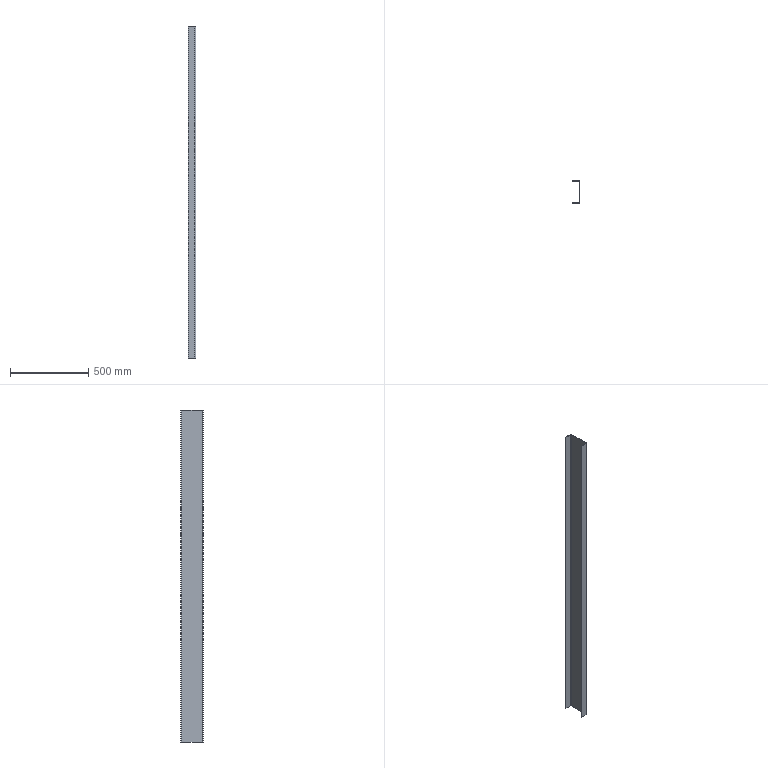Part | SolidWorks | features Extrusion 1 | 1 solid | 14 faces | box 50 x 145 x 2124 mm | volume 1969794 mm3 | plane 10 | cylinder 4 | commonest cylinder face diameters 8 x2 16 x2
STEP:
#1=CARTESIAN_POINT('',(-50.,-68.5,-1062.));
#2=VERTEX_POINT('',#1);
#3=CARTESIAN_POINT('',(-50.,-72.5,-1062.));
#4=VERTEX_POINT('',#3);
#5=CARTESIAN_POINT('',(-50.,-68.5,-1062.));
#6=DIRECTION('',(0.,-1.,0.));
#7=VECTOR('',#6,1000.);
#8=LINE('',#5,#7);
#9=EDGE_CURVE('',#2,#4,#8,.T.);
#10=ORIENTED_EDGE('',*,*,#9,.T.);
#11=CARTESIAN_POINT('',(-50.,-72.5,1062.));
#12=VERTEX_POINT('',#11);
#13=CARTESIAN_POINT('',(-50.,-72.5,1062.));
#14=DIRECTION('',(0.,0.,-1.));
#15=VECTOR('',#14,1000.);
#16=LINE('',#13,#15);
#17=EDGE_CURVE('',#12,#4,#16,.T.);
#18=ORIENTED_EDGE('',*,*,#17,.F.);
#19=CARTESIAN_POINT('',(-50.,-68.5,1062.));
#20=VERTEX_POINT('',#19);
#21=CARTESIAN_POINT('',(-50.,-68.5,1062.));
#22=DIRECTION('',(0.,-1.,0.));
#23=VECTOR('',#22,1000.);
#24=LINE('',#21,#23);
#25=EDGE_CURVE('',#20,#12,#24,.T.);
#26=ORIENTED_EDGE('',*,*,#25,.F.);
#27=CARTESIAN_POINT('',(-50.,-68.5,1062.));
#28=DIRECTION('',(0.,0.,-1.));
#29=VECTOR('',#28,1000.);
#30=LINE('',#27,#29);
#31=EDGE_CURVE('',#20,#2,#30,.T.);
#32=ORIENTED_EDGE('',*,*,#31,.T.);
#33=EDGE_LOOP('',(#10,#18,#26,#32));
#34=FACE_OUTER_BOUND('',#33,.T.);
#35=CARTESIAN_POINT('',(-50.,-68.5,1062.));
#36=DIRECTION('',(1.,0.,0.));
#37=DIRECTION('',(0.,0.,-1.));
#38=AXIS2_PLACEMENT_3D('',#35,#36,#37);
#39=PLANE('',#38);
#40=ADVANCED_FACE('',(#34),#39,.F.);
#41=CARTESIAN_POINT('',(-8.,-72.5,-1062.));
#42=VERTEX_POINT('',#41);
#43=CARTESIAN_POINT('',(-50.,-72.5,-1062.));
#44=DIRECTION('',(1.,0.,0.));
#45=VECTOR('',#44,1000.);
#46=LINE('',#43,#45);
#47=EDGE_CURVE('',#4,#42,#46,.T.);
#48=ORIENTED_EDGE('',*,*,#47,.T.);
#49=CARTESIAN_POINT('',(-8.,-72.5,1062.));
#50=VERTEX_POINT('',#49);
#51=CARTESIAN_POINT('',(-8.,-72.5,1062.));
#52=DIRECTION('',(0.,0.,-1.));
#53=VECTOR('',#52,1000.);
#54=LINE('',#51,#53);
#55=EDGE_CURVE('',#50,#42,#54,.T.);
#56=ORIENTED_EDGE('',*,*,#55,.F.);
#57=CARTESIAN_POINT('',(-50.,-72.5,1062.));
#58=DIRECTION('',(1.,0.,0.));
#59=VECTOR('',#58,1000.);
#60=LINE('',#57,#59);
#61=EDGE_CURVE('',#12,#50,#60,.T.);
#62=ORIENTED_EDGE('',*,*,#61,.F.);
#63=ORIENTED_EDGE('',*,*,#17,.T.);
#64=EDGE_LOOP('',(#48,#56,#62,#63));
#65=FACE_OUTER_BOUND('',#64,.T.);
#66=CARTESIAN_POINT('',(-50.,-72.5,1062.));
#67=DIRECTION('',(0.,1.,0.));
#68=DIRECTION('',(0.,0.,1.));
#69=AXIS2_PLACEMENT_3D('',#66,#67,#68);
#70=PLANE('',#69);
#71=ADVANCED_FACE('',(#65),#70,.F.);
#72=CARTESIAN_POINT('',(0.,-64.5,-1062.));
#73=VERTEX_POINT('',#72);
#74=CARTESIAN_POINT('',(-8.,-64.5,-1062.));
#75=DIRECTION('',(0.,0.,1.));
#76=DIRECTION('',(1.,0.,0.));
#77=AXIS2_PLACEMENT_3D('',#74,#75,#76);
#78=CIRCLE('',#77,8.);
#79=EDGE_CURVE('',#42,#73,#78,.T.);
#80=ORIENTED_EDGE('',*,*,#79,.T.);
#81=CARTESIAN_POINT('',(0.,-64.5,1062.));
#82=VERTEX_POINT('',#81);
#83=CARTESIAN_POINT('',(0.,-64.5,1062.));
#84=DIRECTION('',(0.,0.,-1.));
#85=VECTOR('',#84,1000.);
#86=LINE('',#83,#85);
#87=EDGE_CURVE('',#82,#73,#86,.T.);
#88=ORIENTED_EDGE('',*,*,#87,.F.);
#89=CARTESIAN_POINT('',(-8.,-64.5,1062.));
#90=DIRECTION('',(0.,0.,1.));
#91=DIRECTION('',(1.,0.,0.));
#92=AXIS2_PLACEMENT_3D('',#89,#90,#91);
#93=CIRCLE('',#92,8.);
#94=EDGE_CURVE('',#50,#82,#93,.T.);
#95=ORIENTED_EDGE('',*,*,#94,.F.);
#96=ORIENTED_EDGE('',*,*,#55,.T.);
#97=EDGE_LOOP('',(#80,#88,#95,#96));
#98=FACE_OUTER_BOUND('',#97,.T.);
#99=CARTESIAN_POINT('',(-8.,-64.5,1062.));
#100=DIRECTION('',(0.,0.,-1.));
#101=DIRECTION('',(-1.,0.,0.));
#102=AXIS2_PLACEMENT_3D('',#99,#100,#101);
#103=CYLINDRICAL_SURFACE('',#102,8.);
#104=ADVANCED_FACE('',(#98),#103,.T.);
#105=CARTESIAN_POINT('',(0.,64.5,-1062.));
#106=VERTEX_POINT('',#105);
#107=CARTESIAN_POINT('',(0.,-64.5,-1062.));
#108=DIRECTION('',(0.,1.,0.));
#109=VECTOR('',#108,1000.);
#110=LINE('',#107,#109);
#111=EDGE_CURVE('',#73,#106,#110,.T.);
#112=ORIENTED_EDGE('',*,*,#111,.T.);
#113=CARTESIAN_POINT('',(0.,64.5,1062.));
#114=VERTEX_POINT('',#113);
#115=CARTESIAN_POINT('',(0.,64.5,1062.));
#116=DIRECTION('',(0.,0.,-1.));
#117=VECTOR('',#116,1000.);
#118=LINE('',#115,#117);
#119=EDGE_CURVE('',#114,#106,#118,.T.);
#120=ORIENTED_EDGE('',*,*,#119,.F.);
#121=CARTESIAN_POINT('',(0.,-64.5,1062.));
#122=DIRECTION('',(0.,1.,0.));
#123=VECTOR('',#122,1000.);
#124=LINE('',#121,#123);
#125=EDGE_CURVE('',#82,#114,#124,.T.);
#126=ORIENTED_EDGE('',*,*,#125,.F.);
#127=ORIENTED_EDGE('',*,*,#87,.T.);
#128=EDGE_LOOP('',(#112,#120,#126,#127));
#129=FACE_OUTER_BOUND('',#128,.T.);
#130=CARTESIAN_POINT('',(0.,-64.5,1062.));
#131=DIRECTION('',(-1.,0.,0.));
#132=DIRECTION('',(0.,0.,1.));
#133=AXIS2_PLACEMENT_3D('',#130,#131,#132);
#134=PLANE('',#133);
#135=ADVANCED_FACE('',(#129),#134,.F.);
#136=CARTESIAN_POINT('',(-8.,72.5,-1062.));
#137=VERTEX_POINT('',#136);
#138=CARTESIAN_POINT('',(-8.,64.5,-1062.));
#139=DIRECTION('',(0.,0.,1.));
#140=DIRECTION('',(1.,0.,0.));
#141=AXIS2_PLACEMENT_3D('',#138,#139,#140);
#142=CIRCLE('',#141,8.);
#143=EDGE_CURVE('',#106,#137,#142,.T.);
#144=ORIENTED_EDGE('',*,*,#143,.T.);
#145=CARTESIAN_POINT('',(-8.,72.5,1062.));
#146=VERTEX_POINT('',#145);
#147=CARTESIAN_POINT('',(-8.,72.5,1062.));
#148=DIRECTION('',(0.,0.,-1.));
#149=VECTOR('',#148,1000.);
#150=LINE('',#147,#149);
#151=EDGE_CURVE('',#146,#137,#150,.T.);
#152=ORIENTED_EDGE('',*,*,#151,.F.);
#153=CARTESIAN_POINT('',(-8.,64.5,1062.));
#154=DIRECTION('',(0.,0.,1.));
#155=DIRECTION('',(1.,0.,0.));
#156=AXIS2_PLACEMENT_3D('',#153,#154,#155);
#157=CIRCLE('',#156,8.);
#158=EDGE_CURVE('',#114,#146,#157,.T.);
#159=ORIENTED_EDGE('',*,*,#158,.F.);
#160=ORIENTED_EDGE('',*,*,#119,.T.);
#161=EDGE_LOOP('',(#144,#152,#159,#160));
#162=FACE_OUTER_BOUND('',#161,.T.);
#163=CARTESIAN_POINT('',(-8.,64.5,1062.));
#164=DIRECTION('',(0.,0.,-1.));
#165=DIRECTION('',(-1.,0.,0.));
#166=AXIS2_PLACEMENT_3D('',#163,#164,#165);
#167=CYLINDRICAL_SURFACE('',#166,8.);
#168=ADVANCED_FACE('',(#162),#167,.T.);
#169=CARTESIAN_POINT('',(-50.,72.5,-1062.));
#170=VERTEX_POINT('',#169);
#171=CARTESIAN_POINT('',(-8.,72.5,-1062.));
#172=DIRECTION('',(-1.,0.,0.));
#173=VECTOR('',#172,1000.);
#174=LINE('',#171,#173);
#175=EDGE_CURVE('',#137,#170,#174,.T.);
#176=ORIENTED_EDGE('',*,*,#175,.T.);
#177=CARTESIAN_POINT('',(-50.,72.5,1062.));
#178=VERTEX_POINT('',#177);
#179=CARTESIAN_POINT('',(-50.,72.5,1062.));
#180=DIRECTION('',(0.,0.,-1.));
#181=VECTOR('',#180,1000.);
#182=LINE('',#179,#181);
#183=EDGE_CURVE('',#178,#170,#182,.T.);
#184=ORIENTED_EDGE('',*,*,#183,.F.);
#185=CARTESIAN_POINT('',(-8.,72.5,1062.));
#186=DIRECTION('',(-1.,0.,0.));
#187=VECTOR('',#186,1000.);
#188=LINE('',#185,#187);
#189=EDGE_CURVE('',#146,#178,#188,.T.);
#190=ORIENTED_EDGE('',*,*,#189,.F.);
#191=ORIENTED_EDGE('',*,*,#151,.T.);
#192=EDGE_LOOP('',(#176,#184,#190,#191));
#193=FACE_OUTER_BOUND('',#192,.T.);
#194=CARTESIAN_POINT('',(-8.,72.5,1062.));
#195=DIRECTION('',(0.,-1.,0.));
#196=DIRECTION('',(1.,0.,0.));
#197=AXIS2_PLACEMENT_3D('',#194,#195,#196);
#198=PLANE('',#197);
#199=ADVANCED_FACE('',(#193),#198,.F.);
#200=CARTESIAN_POINT('',(-50.,68.5,-1062.));
#201=VERTEX_POINT('',#200);
#202=CARTESIAN_POINT('',(-50.,72.5,-1062.));
#203=DIRECTION('',(0.,-1.,0.));
#204=VECTOR('',#203,1000.);
#205=LINE('',#202,#204);
#206=EDGE_CURVE('',#170,#201,#205,.T.);
#207=ORIENTED_EDGE('',*,*,#206,.T.);
#208=CARTESIAN_POINT('',(-50.,68.5,1062.));
#209=VERTEX_POINT('',#208);
#210=CARTESIAN_POINT('',(-50.,68.5,1062.));
#211=DIRECTION('',(0.,0.,-1.));
#212=VECTOR('',#211,1000.);
#213=LINE('',#210,#212);
#214=EDGE_CURVE('',#209,#201,#213,.T.);
#215=ORIENTED_EDGE('',*,*,#214,.F.);
#216=CARTESIAN_POINT('',(-50.,72.5,1062.));
#217=DIRECTION('',(0.,-1.,0.));
#218=VECTOR('',#217,1000.);
#219=LINE('',#216,#218);
#220=EDGE_CURVE('',#178,#209,#219,.T.);
#221=ORIENTED_EDGE('',*,*,#220,.F.);
#222=ORIENTED_EDGE('',*,*,#183,.T.);
#223=EDGE_LOOP('',(#207,#215,#221,#222));
#224=FACE_OUTER_BOUND('',#223,.T.);
#225=CARTESIAN_POINT('',(-50.,72.5,1062.));
#226=DIRECTION('',(1.,0.,0.));
#227=DIRECTION('',(0.,0.,-1.));
#228=AXIS2_PLACEMENT_3D('',#225,#226,#227);
#229=PLANE('',#228);
#230=ADVANCED_FACE('',(#224),#229,.F.);
#231=CARTESIAN_POINT('',(-8.,68.5,-1062.));
#232=VERTEX_POINT('',#231);
#233=CARTESIAN_POINT('',(-50.,68.5,-1062.));
#234=DIRECTION('',(1.,0.,0.));
#235=VECTOR('',#234,1000.);
#236=LINE('',#233,#235);
#237=EDGE_CURVE('',#201,#232,#236,.T.);
#238=ORIENTED_EDGE('',*,*,#237,.T.);
#239=CARTESIAN_POINT('',(-8.,68.5,1062.));
#240=VERTEX_POINT('',#239);
#241=CARTESIAN_POINT('',(-8.,68.5,1062.));
#242=DIRECTION('',(0.,0.,-1.));
#243=VECTOR('',#242,1000.);
#244=LINE('',#241,#243);
#245=EDGE_CURVE('',#240,#232,#244,.T.);
#246=ORIENTED_EDGE('',*,*,#245,.F.);
#247=CARTESIAN_POINT('',(-50.,68.5,1062.));
#248=DIRECTION('',(1.,0.,0.));
#249=VECTOR('',#248,1000.);
#250=LINE('',#247,#249);
#251=EDGE_CURVE('',#209,#240,#250,.T.);
#252=ORIENTED_EDGE('',*,*,#251,.F.);
#253=ORIENTED_EDGE('',*,*,#214,.T.);
#254=EDGE_LOOP('',(#238,#246,#252,#253));
#255=FACE_OUTER_BOUND('',#254,.T.);
#256=CARTESIAN_POINT('',(-50.,68.5,1062.));
#257=DIRECTION('',(0.,1.,0.));
#258=DIRECTION('',(0.,0.,1.));
#259=AXIS2_PLACEMENT_3D('',#256,#257,#258);
#260=PLANE('',#259);
#261=ADVANCED_FACE('',(#255),#260,.F.);
#262=CARTESIAN_POINT('',(-4.,64.5,-1062.));
#263=VERTEX_POINT('',#262);
#264=CARTESIAN_POINT('',(-8.,64.5,-1062.));
#265=DIRECTION('',(0.,0.,-1.));
#266=DIRECTION('',(1.,0.,0.));
#267=AXIS2_PLACEMENT_3D('',#264,#265,#266);
#268=CIRCLE('',#267,4.);
#269=EDGE_CURVE('',#232,#263,#268,.T.);
#270=ORIENTED_EDGE('',*,*,#269,.T.);
#271=CARTESIAN_POINT('',(-4.,64.5,1062.));
#272=VERTEX_POINT('',#271);
#273=CARTESIAN_POINT('',(-4.,64.5,1062.));
#274=DIRECTION('',(0.,0.,-1.));
#275=VECTOR('',#274,1000.);
#276=LINE('',#273,#275);
#277=EDGE_CURVE('',#272,#263,#276,.T.);
#278=ORIENTED_EDGE('',*,*,#277,.F.);
#279=CARTESIAN_POINT('',(-8.,64.5,1062.));
#280=DIRECTION('',(0.,0.,-1.));
#281=DIRECTION('',(1.,0.,0.));
#282=AXIS2_PLACEMENT_3D('',#279,#280,#281);
#283=CIRCLE('',#282,4.);
#284=EDGE_CURVE('',#240,#272,#283,.T.);
#285=ORIENTED_EDGE('',*,*,#284,.F.);
#286=ORIENTED_EDGE('',*,*,#245,.T.);
#287=EDGE_LOOP('',(#270,#278,#285,#286));
#288=FACE_OUTER_BOUND('',#287,.T.);
#289=CARTESIAN_POINT('',(-8.,64.5,1062.));
#290=DIRECTION('',(0.,0.,-1.));
#291=DIRECTION('',(-1.,0.,0.));
#292=AXIS2_PLACEMENT_3D('',#289,#290,#291);
#293=CYLINDRICAL_SURFACE('',#292,4.);
#294=ADVANCED_FACE('',(#288),#293,.F.);
#295=CARTESIAN_POINT('',(-4.,-64.5,-1062.));
#296=VERTEX_POINT('',#295);
#297=CARTESIAN_POINT('',(-4.,64.5,-1062.));
#298=DIRECTION('',(0.,-1.,0.));
#299=VECTOR('',#298,1000.);
#300=LINE('',#297,#299);
#301=EDGE_CURVE('',#263,#296,#300,.T.);
#302=ORIENTED_EDGE('',*,*,#301,.T.);
#303=CARTESIAN_POINT('',(-4.,-64.5,1062.));
#304=VERTEX_POINT('',#303);
#305=CARTESIAN_POINT('',(-4.,-64.5,1062.));
#306=DIRECTION('',(0.,0.,-1.));
#307=VECTOR('',#306,1000.);
#308=LINE('',#305,#307);
#309=EDGE_CURVE('',#304,#296,#308,.T.);
#310=ORIENTED_EDGE('',*,*,#309,.F.);
#311=CARTESIAN_POINT('',(-4.,64.5,1062.));
#312=DIRECTION('',(0.,-1.,0.));
#313=VECTOR('',#312,1000.);
#314=LINE('',#311,#313);
#315=EDGE_CURVE('',#272,#304,#314,.T.);
#316=ORIENTED_EDGE('',*,*,#315,.F.);
#317=ORIENTED_EDGE('',*,*,#277,.T.);
#318=EDGE_LOOP('',(#302,#310,#316,#317));
#319=FACE_OUTER_BOUND('',#318,.T.);
#320=CARTESIAN_POINT('',(-4.,64.5,1062.));
#321=DIRECTION('',(1.,0.,0.));
#322=DIRECTION('',(0.,1.,0.));
#323=AXIS2_PLACEMENT_3D('',#320,#321,#322);
#324=PLANE('',#323);
#325=ADVANCED_FACE('',(#319),#324,.F.);
#326=CARTESIAN_POINT('',(-8.,-68.5,-1062.));
#327=VERTEX_POINT('',#326);
#328=CARTESIAN_POINT('',(-8.,-64.5,-1062.));
#329=DIRECTION('',(0.,0.,-1.));
#330=DIRECTION('',(1.,0.,0.));
#331=AXIS2_PLACEMENT_3D('',#328,#329,#330);
#332=CIRCLE('',#331,4.);
#333=EDGE_CURVE('',#296,#327,#332,.T.);
#334=ORIENTED_EDGE('',*,*,#333,.T.);
#335=CARTESIAN_POINT('',(-8.,-68.5,1062.));
#336=VERTEX_POINT('',#335);
#337=CARTESIAN_POINT('',(-8.,-68.5,1062.));
#338=DIRECTION('',(0.,0.,-1.));
#339=VECTOR('',#338,1000.);
#340=LINE('',#337,#339);
#341=EDGE_CURVE('',#336,#327,#340,.T.);
#342=ORIENTED_EDGE('',*,*,#341,.F.);
#343=CARTESIAN_POINT('',(-8.,-64.5,1062.));
#344=DIRECTION('',(0.,0.,-1.));
#345=DIRECTION('',(1.,0.,0.));
#346=AXIS2_PLACEMENT_3D('',#343,#344,#345);
#347=CIRCLE('',#346,4.);
#348=EDGE_CURVE('',#304,#336,#347,.T.);
#349=ORIENTED_EDGE('',*,*,#348,.F.);
#350=ORIENTED_EDGE('',*,*,#309,.T.);
#351=EDGE_LOOP('',(#334,#342,#349,#350));
#352=FACE_OUTER_BOUND('',#351,.T.);
#353=CARTESIAN_POINT('',(-8.,-64.5,1062.));
#354=DIRECTION('',(0.,0.,-1.));
#355=DIRECTION('',(-1.,0.,0.));
#356=AXIS2_PLACEMENT_3D('',#353,#354,#355);
#357=CYLINDRICAL_SURFACE('',#356,4.);
#358=ADVANCED_FACE('',(#352),#357,.F.);
#359=CARTESIAN_POINT('',(-8.,-68.5,-1062.));
#360=DIRECTION('',(-1.,0.,0.));
#361=VECTOR('',#360,1000.);
#362=LINE('',#359,#361);
#363=EDGE_CURVE('',#327,#2,#362,.T.);
#364=ORIENTED_EDGE('',*,*,#363,.T.);
#365=ORIENTED_EDGE('',*,*,#31,.F.);
#366=CARTESIAN_POINT('',(-8.,-68.5,1062.));
#367=DIRECTION('',(-1.,0.,0.));
#368=VECTOR('',#367,1000.);
#369=LINE('',#366,#368);
#370=EDGE_CURVE('',#336,#20,#369,.T.);
#371=ORIENTED_EDGE('',*,*,#370,.F.);
#372=ORIENTED_EDGE('',*,*,#341,.T.);
#373=EDGE_LOOP('',(#364,#365,#371,#372));
#374=FACE_OUTER_BOUND('',#373,.T.);
#375=CARTESIAN_POINT('',(-8.,-68.5,1062.));
#376=DIRECTION('',(0.,-1.,0.));
#377=DIRECTION('',(0.,0.,-1.));
#378=AXIS2_PLACEMENT_3D('',#375,#376,#377);
#379=PLANE('',#378);
#380=ADVANCED_FACE('',(#374),#379,.F.);
#381=ORIENTED_EDGE('',*,*,#25,.T.);
#382=ORIENTED_EDGE('',*,*,#61,.T.);
#383=ORIENTED_EDGE('',*,*,#94,.T.);
#384=ORIENTED_EDGE('',*,*,#125,.T.);
#385=ORIENTED_EDGE('',*,*,#158,.T.);
#386=ORIENTED_EDGE('',*,*,#189,.T.);
#387=ORIENTED_EDGE('',*,*,#220,.T.);
#388=ORIENTED_EDGE('',*,*,#251,.T.);
#389=ORIENTED_EDGE('',*,*,#284,.T.);
#390=ORIENTED_EDGE('',*,*,#315,.T.);
#391=ORIENTED_EDGE('',*,*,#348,.T.);
#392=ORIENTED_EDGE('',*,*,#370,.T.);
#393=EDGE_LOOP('',(#381,#382,#383,#384,#385,#386,#387,#388,#389,#390,#391,#392));
#394=FACE_OUTER_BOUND('',#393,.T.);
#395=CARTESIAN_POINT('',(-8.,-64.5,1062.));
#396=DIRECTION('',(0.,0.,1.));
#397=DIRECTION('',(1.,0.,0.));
#398=AXIS2_PLACEMENT_3D('',#395,#396,#397);
#399=PLANE('',#398);
#400=ADVANCED_FACE('',(#394),#399,.T.);
#401=ORIENTED_EDGE('',*,*,#9,.F.);
#402=ORIENTED_EDGE('',*,*,#363,.F.);
#403=ORIENTED_EDGE('',*,*,#333,.F.);
#404=ORIENTED_EDGE('',*,*,#301,.F.);
#405=ORIENTED_EDGE('',*,*,#269,.F.);
#406=ORIENTED_EDGE('',*,*,#237,.F.);
#407=ORIENTED_EDGE('',*,*,#206,.F.);
#408=ORIENTED_EDGE('',*,*,#175,.F.);
#409=ORIENTED_EDGE('',*,*,#143,.F.);
#410=ORIENTED_EDGE('',*,*,#111,.F.);
#411=ORIENTED_EDGE('',*,*,#79,.F.);
#412=ORIENTED_EDGE('',*,*,#47,.F.);
#413=EDGE_LOOP('',(#401,#402,#403,#404,#405,#406,#407,#408,#409,#410,#411,#412));
#414=FACE_OUTER_BOUND('',#413,.T.);
#415=CARTESIAN_POINT('',(-8.,-64.5,-1062.));
#416=DIRECTION('',(0.,0.,1.));
#417=DIRECTION('',(1.,0.,0.));
#418=AXIS2_PLACEMENT_3D('',#415,#416,#417);
#419=PLANE('',#418);
#420=ADVANCED_FACE('',(#414),#419,.F.);
#421=CLOSED_SHELL('',(#40,#71,#104,#135,#168,#199,#230,#261,#294,#325,#358,#380,#400,#420));
#422=MANIFOLD_SOLID_BREP('',#421);
#423=CARTESIAN_POINT('',(0.,0.,0.));
#424=DIRECTION('',(0.,0.,1.));
#425=DIRECTION('',(1.,0.,0.));
#426=AXIS2_PLACEMENT_3D('',#423,#424,#425);
#427=(LENGTH_UNIT()NAMED_UNIT(*)SI_UNIT(.MILLI.,.METRE.));
#428=UNCERTAINTY_MEASURE_WITH_UNIT(LENGTH_MEASURE(0.00001),#427,'','');
#429=(NAMED_UNIT(*)PLANE_ANGLE_UNIT()SI_UNIT($,.RADIAN.));
#430=(NAMED_UNIT(*)SI_UNIT($,.STERADIAN.)SOLID_ANGLE_UNIT());
#431=(GEOMETRIC_REPRESENTATION_CONTEXT(3)GLOBAL_UNCERTAINTY_ASSIGNED_CONTEXT((#428))GLOBAL_UNIT_ASSIGNED_CONTEXT((#427,#429,#430))REPRESENTATION_CONTEXT('',''));
#432=ADVANCED_BREP_SHAPE_REPRESENTATION('',(#422,#426),#431);